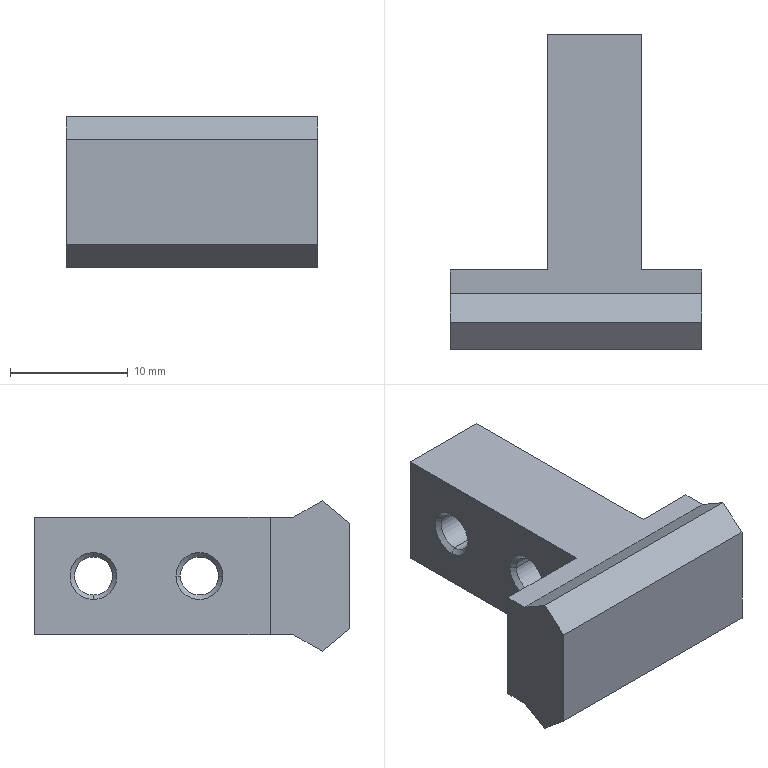Part | SolidWorks | features BaseBody 1 | 1 solid | 26 faces | box 21.4 x 26.74 x 12.8 mm | volume 3023 mm3 | plane 14 | cone 8 | cylinder 4 | commonest cylinder face diameters 3.242 x4
STEP:
#1=CARTESIAN_POINT('',(8.629,19.44,1.621));
#2=VERTEX_POINT('',#1);
#3=CARTESIAN_POINT('',(8.629,19.44,-1.621));
#4=VERTEX_POINT('',#3);
#5=CARTESIAN_POINT('',(8.629,19.44,0.));
#6=DIRECTION('',(1.,0.,0.));
#7=DIRECTION('',(0.,0.,-1.));
#8=AXIS2_PLACEMENT_3D('',#5,#6,#7);
#9=CIRCLE('',#8,1.621);
#10=EDGE_CURVE('',#2,#4,#9,.T.);
#11=ORIENTED_EDGE('',*,*,#10,.T.);
#12=CARTESIAN_POINT('',(8.25,19.44,-2.));
#13=VERTEX_POINT('',#12);
#14=CARTESIAN_POINT('',(8.25,19.44,-2.));
#15=DIRECTION('',(-0.7071,0.,-0.7071));
#16=VECTOR('',#15,1000.);
#17=LINE('',#14,#16);
#18=EDGE_CURVE('',#4,#13,#17,.T.);
#19=ORIENTED_EDGE('',*,*,#18,.T.);
#20=CARTESIAN_POINT('',(8.25,19.44,2.));
#21=VERTEX_POINT('',#20);
#22=CARTESIAN_POINT('',(8.25,19.44,0.));
#23=DIRECTION('',(1.,0.,0.));
#24=DIRECTION('',(0.,0.,-1.));
#25=AXIS2_PLACEMENT_3D('',#22,#23,#24);
#26=CIRCLE('',#25,2.);
#27=EDGE_CURVE('',#21,#13,#26,.T.);
#28=ORIENTED_EDGE('',*,*,#27,.F.);
#29=CARTESIAN_POINT('',(8.25,19.44,2.));
#30=DIRECTION('',(-0.7071,0.,0.7071));
#31=VECTOR('',#30,1000.);
#32=LINE('',#29,#31);
#33=EDGE_CURVE('',#2,#21,#32,.T.);
#34=ORIENTED_EDGE('',*,*,#33,.F.);
#35=EDGE_LOOP('',(#11,#19,#28,#34));
#36=FACE_OUTER_BOUND('',#35,.T.);
#37=CARTESIAN_POINT('',(8.25,19.44,0.));
#38=DIRECTION('',(-1.,0.,0.));
#39=DIRECTION('',(0.,0.,1.));
#40=AXIS2_PLACEMENT_3D('',#37,#38,#39);
#41=CONICAL_SURFACE('',#40,2.,0.7854);
#42=ADVANCED_FACE('',(#36),#41,.F.);
#43=ORIENTED_EDGE('',*,*,#10,.F.);
#44=CARTESIAN_POINT('',(15.871,19.44,1.621));
#45=VERTEX_POINT('',#44);
#46=CARTESIAN_POINT('',(16.25,19.44,1.621));
#47=DIRECTION('',(1.,0.,0.));
#48=VECTOR('',#47,1000.);
#49=LINE('',#46,#48);
#50=EDGE_CURVE('',#2,#45,#49,.T.);
#51=ORIENTED_EDGE('',*,*,#50,.T.);
#52=CARTESIAN_POINT('',(15.871,19.44,-1.621));
#53=VERTEX_POINT('',#52);
#54=CARTESIAN_POINT('',(15.871,19.44,0.));
#55=DIRECTION('',(1.,0.,0.));
#56=DIRECTION('',(0.,0.,-1.));
#57=AXIS2_PLACEMENT_3D('',#54,#55,#56);
#58=CIRCLE('',#57,1.621);
#59=EDGE_CURVE('',#45,#53,#58,.T.);
#60=ORIENTED_EDGE('',*,*,#59,.T.);
#61=CARTESIAN_POINT('',(16.25,19.44,-1.621));
#62=DIRECTION('',(1.,0.,0.));
#63=VECTOR('',#62,1000.);
#64=LINE('',#61,#63);
#65=EDGE_CURVE('',#4,#53,#64,.T.);
#66=ORIENTED_EDGE('',*,*,#65,.F.);
#67=EDGE_LOOP('',(#43,#51,#60,#66));
#68=FACE_OUTER_BOUND('',#67,.T.);
#69=CARTESIAN_POINT('',(16.25,19.44,0.));
#70=DIRECTION('',(1.,0.,0.));
#71=DIRECTION('',(0.,0.,-1.));
#72=AXIS2_PLACEMENT_3D('',#69,#70,#71);
#73=CYLINDRICAL_SURFACE('',#72,1.621);
#74=ADVANCED_FACE('',(#68),#73,.F.);
#75=ORIENTED_EDGE('',*,*,#59,.F.);
#76=CARTESIAN_POINT('',(16.25,19.44,2.));
#77=VERTEX_POINT('',#76);
#78=CARTESIAN_POINT('',(15.871,19.44,1.621));
#79=DIRECTION('',(0.7071,0.,0.7071));
#80=VECTOR('',#79,1000.);
#81=LINE('',#78,#80);
#82=EDGE_CURVE('',#45,#77,#81,.T.);
#83=ORIENTED_EDGE('',*,*,#82,.T.);
#84=CARTESIAN_POINT('',(16.25,19.44,-2.));
#85=VERTEX_POINT('',#84);
#86=CARTESIAN_POINT('',(16.25,19.44,0.));
#87=DIRECTION('',(1.,0.,0.));
#88=DIRECTION('',(0.,0.,-1.));
#89=AXIS2_PLACEMENT_3D('',#86,#87,#88);
#90=CIRCLE('',#89,2.);
#91=EDGE_CURVE('',#77,#85,#90,.T.);
#92=ORIENTED_EDGE('',*,*,#91,.T.);
#93=CARTESIAN_POINT('',(15.871,19.44,-1.621));
#94=DIRECTION('',(0.7071,0.,-0.7071));
#95=VECTOR('',#94,1000.);
#96=LINE('',#93,#95);
#97=EDGE_CURVE('',#53,#85,#96,.T.);
#98=ORIENTED_EDGE('',*,*,#97,.F.);
#99=EDGE_LOOP('',(#75,#83,#92,#98));
#100=FACE_OUTER_BOUND('',#99,.T.);
#101=CARTESIAN_POINT('',(15.871,19.44,0.));
#102=DIRECTION('',(1.,0.,0.));
#103=DIRECTION('',(0.,0.,-1.));
#104=AXIS2_PLACEMENT_3D('',#101,#102,#103);
#105=CONICAL_SURFACE('',#104,1.621,0.7854);
#106=ADVANCED_FACE('',(#100),#105,.F.);
#107=CARTESIAN_POINT('',(8.629,8.819,0.));
#108=VERTEX_POINT('',#107);
#109=CARTESIAN_POINT('',(8.629,12.061,0.));
#110=VERTEX_POINT('',#109);
#111=CARTESIAN_POINT('',(8.629,10.44,0.));
#112=DIRECTION('',(1.,0.,0.));
#113=DIRECTION('',(0.,1.,0.));
#114=AXIS2_PLACEMENT_3D('',#111,#112,#113);
#115=CIRCLE('',#114,1.621);
#116=EDGE_CURVE('',#108,#110,#115,.T.);
#117=ORIENTED_EDGE('',*,*,#116,.T.);
#118=CARTESIAN_POINT('',(8.25,12.44,0.));
#119=VERTEX_POINT('',#118);
#120=CARTESIAN_POINT('',(8.25,12.44,0.));
#121=DIRECTION('',(-0.7071,0.7071,0.));
#122=VECTOR('',#121,1000.);
#123=LINE('',#120,#122);
#124=EDGE_CURVE('',#110,#119,#123,.T.);
#125=ORIENTED_EDGE('',*,*,#124,.T.);
#126=CARTESIAN_POINT('',(8.25,8.44,0.));
#127=VERTEX_POINT('',#126);
#128=CARTESIAN_POINT('',(8.25,10.44,0.));
#129=DIRECTION('',(1.,0.,0.));
#130=DIRECTION('',(0.,1.,0.));
#131=AXIS2_PLACEMENT_3D('',#128,#129,#130);
#132=CIRCLE('',#131,2.);
#133=EDGE_CURVE('',#127,#119,#132,.T.);
#134=ORIENTED_EDGE('',*,*,#133,.F.);
#135=CARTESIAN_POINT('',(8.25,8.44,0.));
#136=DIRECTION('',(-0.7071,-0.7071,0.));
#137=VECTOR('',#136,1000.);
#138=LINE('',#135,#137);
#139=EDGE_CURVE('',#108,#127,#138,.T.);
#140=ORIENTED_EDGE('',*,*,#139,.F.);
#141=EDGE_LOOP('',(#117,#125,#134,#140));
#142=FACE_OUTER_BOUND('',#141,.T.);
#143=CARTESIAN_POINT('',(8.25,10.44,0.));
#144=DIRECTION('',(-1.,0.,0.));
#145=DIRECTION('',(0.,-1.,0.));
#146=AXIS2_PLACEMENT_3D('',#143,#144,#145);
#147=CONICAL_SURFACE('',#146,2.,0.7854);
#148=ADVANCED_FACE('',(#142),#147,.F.);
#149=ORIENTED_EDGE('',*,*,#116,.F.);
#150=CARTESIAN_POINT('',(15.871,8.819,0.));
#151=VERTEX_POINT('',#150);
#152=CARTESIAN_POINT('',(16.25,8.819,0.));
#153=DIRECTION('',(1.,0.,0.));
#154=VECTOR('',#153,1000.);
#155=LINE('',#152,#154);
#156=EDGE_CURVE('',#108,#151,#155,.T.);
#157=ORIENTED_EDGE('',*,*,#156,.T.);
#158=CARTESIAN_POINT('',(15.871,12.061,0.));
#159=VERTEX_POINT('',#158);
#160=CARTESIAN_POINT('',(15.871,10.44,0.));
#161=DIRECTION('',(1.,0.,0.));
#162=DIRECTION('',(0.,1.,0.));
#163=AXIS2_PLACEMENT_3D('',#160,#161,#162);
#164=CIRCLE('',#163,1.621);
#165=EDGE_CURVE('',#151,#159,#164,.T.);
#166=ORIENTED_EDGE('',*,*,#165,.T.);
#167=CARTESIAN_POINT('',(16.25,12.061,0.));
#168=DIRECTION('',(1.,0.,0.));
#169=VECTOR('',#168,1000.);
#170=LINE('',#167,#169);
#171=EDGE_CURVE('',#110,#159,#170,.T.);
#172=ORIENTED_EDGE('',*,*,#171,.F.);
#173=EDGE_LOOP('',(#149,#157,#166,#172));
#174=FACE_OUTER_BOUND('',#173,.T.);
#175=CARTESIAN_POINT('',(16.25,10.44,0.));
#176=DIRECTION('',(1.,0.,0.));
#177=DIRECTION('',(0.,1.,0.));
#178=AXIS2_PLACEMENT_3D('',#175,#176,#177);
#179=CYLINDRICAL_SURFACE('',#178,1.621);
#180=ADVANCED_FACE('',(#174),#179,.F.);
#181=ORIENTED_EDGE('',*,*,#165,.F.);
#182=CARTESIAN_POINT('',(16.25,8.44,0.));
#183=VERTEX_POINT('',#182);
#184=CARTESIAN_POINT('',(15.871,8.819,0.));
#185=DIRECTION('',(0.7071,-0.7071,0.));
#186=VECTOR('',#185,1000.);
#187=LINE('',#184,#186);
#188=EDGE_CURVE('',#151,#183,#187,.T.);
#189=ORIENTED_EDGE('',*,*,#188,.T.);
#190=CARTESIAN_POINT('',(16.25,12.44,0.));
#191=VERTEX_POINT('',#190);
#192=CARTESIAN_POINT('',(16.25,10.44,0.));
#193=DIRECTION('',(1.,0.,0.));
#194=DIRECTION('',(0.,1.,0.));
#195=AXIS2_PLACEMENT_3D('',#192,#193,#194);
#196=CIRCLE('',#195,2.);
#197=EDGE_CURVE('',#183,#191,#196,.T.);
#198=ORIENTED_EDGE('',*,*,#197,.T.);
#199=CARTESIAN_POINT('',(15.871,12.061,0.));
#200=DIRECTION('',(0.7071,0.7071,0.));
#201=VECTOR('',#200,1000.);
#202=LINE('',#199,#201);
#203=EDGE_CURVE('',#159,#191,#202,.T.);
#204=ORIENTED_EDGE('',*,*,#203,.F.);
#205=EDGE_LOOP('',(#181,#189,#198,#204));
#206=FACE_OUTER_BOUND('',#205,.T.);
#207=CARTESIAN_POINT('',(15.871,10.44,0.));
#208=DIRECTION('',(1.,0.,0.));
#209=DIRECTION('',(0.,1.,0.));
#210=AXIS2_PLACEMENT_3D('',#207,#208,#209);
#211=CONICAL_SURFACE('',#210,1.621,0.7854);
#212=ADVANCED_FACE('',(#206),#211,.F.);
#213=ORIENTED_EDGE('',*,*,#188,.F.);
#214=CARTESIAN_POINT('',(15.871,10.44,0.));
#215=DIRECTION('',(1.,0.,0.));
#216=DIRECTION('',(0.,1.,0.));
#217=AXIS2_PLACEMENT_3D('',#214,#215,#216);
#218=CIRCLE('',#217,1.621);
#219=EDGE_CURVE('',#159,#151,#218,.T.);
#220=ORIENTED_EDGE('',*,*,#219,.F.);
#221=ORIENTED_EDGE('',*,*,#203,.T.);
#222=CARTESIAN_POINT('',(16.25,10.44,0.));
#223=DIRECTION('',(1.,0.,0.));
#224=DIRECTION('',(0.,1.,0.));
#225=AXIS2_PLACEMENT_3D('',#222,#223,#224);
#226=CIRCLE('',#225,2.);
#227=EDGE_CURVE('',#191,#183,#226,.T.);
#228=ORIENTED_EDGE('',*,*,#227,.T.);
#229=EDGE_LOOP('',(#213,#220,#221,#228));
#230=FACE_OUTER_BOUND('',#229,.T.);
#231=CARTESIAN_POINT('',(15.871,10.44,0.));
#232=DIRECTION('',(1.,0.,0.));
#233=DIRECTION('',(0.,1.,0.));
#234=AXIS2_PLACEMENT_3D('',#231,#232,#233);
#235=CONICAL_SURFACE('',#234,1.621,0.7854);
#236=ADVANCED_FACE('',(#230),#235,.F.);
#237=ORIENTED_EDGE('',*,*,#156,.F.);
#238=CARTESIAN_POINT('',(8.629,10.44,0.));
#239=DIRECTION('',(1.,0.,0.));
#240=DIRECTION('',(0.,1.,0.));
#241=AXIS2_PLACEMENT_3D('',#238,#239,#240);
#242=CIRCLE('',#241,1.621);
#243=EDGE_CURVE('',#110,#108,#242,.T.);
#244=ORIENTED_EDGE('',*,*,#243,.F.);
#245=ORIENTED_EDGE('',*,*,#171,.T.);
#246=ORIENTED_EDGE('',*,*,#219,.T.);
#247=EDGE_LOOP('',(#237,#244,#245,#246));
#248=FACE_OUTER_BOUND('',#247,.T.);
#249=CARTESIAN_POINT('',(16.25,10.44,0.));
#250=DIRECTION('',(1.,0.,0.));
#251=DIRECTION('',(0.,1.,0.));
#252=AXIS2_PLACEMENT_3D('',#249,#250,#251);
#253=CYLINDRICAL_SURFACE('',#252,1.621);
#254=ADVANCED_FACE('',(#248),#253,.F.);
#255=ORIENTED_EDGE('',*,*,#124,.F.);
#256=ORIENTED_EDGE('',*,*,#243,.T.);
#257=ORIENTED_EDGE('',*,*,#139,.T.);
#258=CARTESIAN_POINT('',(8.25,10.44,0.));
#259=DIRECTION('',(1.,0.,0.));
#260=DIRECTION('',(0.,1.,0.));
#261=AXIS2_PLACEMENT_3D('',#258,#259,#260);
#262=CIRCLE('',#261,2.);
#263=EDGE_CURVE('',#119,#127,#262,.T.);
#264=ORIENTED_EDGE('',*,*,#263,.F.);
#265=EDGE_LOOP('',(#255,#256,#257,#264));
#266=FACE_OUTER_BOUND('',#265,.T.);
#267=CARTESIAN_POINT('',(8.25,10.44,0.));
#268=DIRECTION('',(-1.,0.,0.));
#269=DIRECTION('',(0.,-1.,0.));
#270=AXIS2_PLACEMENT_3D('',#267,#268,#269);
#271=CONICAL_SURFACE('',#270,2.,0.7854);
#272=ADVANCED_FACE('',(#266),#271,.F.);
#273=ORIENTED_EDGE('',*,*,#82,.F.);
#274=CARTESIAN_POINT('',(15.871,19.44,0.));
#275=DIRECTION('',(1.,0.,0.));
#276=DIRECTION('',(0.,0.,-1.));
#277=AXIS2_PLACEMENT_3D('',#274,#275,#276);
#278=CIRCLE('',#277,1.621);
#279=EDGE_CURVE('',#53,#45,#278,.T.);
#280=ORIENTED_EDGE('',*,*,#279,.F.);
#281=ORIENTED_EDGE('',*,*,#97,.T.);
#282=CARTESIAN_POINT('',(16.25,19.44,0.));
#283=DIRECTION('',(1.,0.,0.));
#284=DIRECTION('',(0.,0.,-1.));
#285=AXIS2_PLACEMENT_3D('',#282,#283,#284);
#286=CIRCLE('',#285,2.);
#287=EDGE_CURVE('',#85,#77,#286,.T.);
#288=ORIENTED_EDGE('',*,*,#287,.T.);
#289=EDGE_LOOP('',(#273,#280,#281,#288));
#290=FACE_OUTER_BOUND('',#289,.T.);
#291=CARTESIAN_POINT('',(15.871,19.44,0.));
#292=DIRECTION('',(1.,0.,0.));
#293=DIRECTION('',(0.,0.,-1.));
#294=AXIS2_PLACEMENT_3D('',#291,#292,#293);
#295=CONICAL_SURFACE('',#294,1.621,0.7854);
#296=ADVANCED_FACE('',(#290),#295,.F.);
#297=ORIENTED_EDGE('',*,*,#50,.F.);
#298=CARTESIAN_POINT('',(8.629,19.44,0.));
#299=DIRECTION('',(1.,0.,0.));
#300=DIRECTION('',(0.,0.,-1.));
#301=AXIS2_PLACEMENT_3D('',#298,#299,#300);
#302=CIRCLE('',#301,1.621);
#303=EDGE_CURVE('',#4,#2,#302,.T.);
#304=ORIENTED_EDGE('',*,*,#303,.F.);
#305=ORIENTED_EDGE('',*,*,#65,.T.);
#306=ORIENTED_EDGE('',*,*,#279,.T.);
#307=EDGE_LOOP('',(#297,#304,#305,#306));
#308=FACE_OUTER_BOUND('',#307,.T.);
#309=CARTESIAN_POINT('',(16.25,19.44,0.));
#310=DIRECTION('',(1.,0.,0.));
#311=DIRECTION('',(0.,0.,-1.));
#312=AXIS2_PLACEMENT_3D('',#309,#310,#311);
#313=CYLINDRICAL_SURFACE('',#312,1.621);
#314=ADVANCED_FACE('',(#308),#313,.F.);
#315=ORIENTED_EDGE('',*,*,#18,.F.);
#316=ORIENTED_EDGE('',*,*,#303,.T.);
#317=ORIENTED_EDGE('',*,*,#33,.T.);
#318=CARTESIAN_POINT('',(8.25,19.44,0.));
#319=DIRECTION('',(1.,0.,0.));
#320=DIRECTION('',(0.,0.,-1.));
#321=AXIS2_PLACEMENT_3D('',#318,#319,#320);
#322=CIRCLE('',#321,2.);
#323=EDGE_CURVE('',#13,#21,#322,.T.);
#324=ORIENTED_EDGE('',*,*,#323,.F.);
#325=EDGE_LOOP('',(#315,#316,#317,#324));
#326=FACE_OUTER_BOUND('',#325,.T.);
#327=CARTESIAN_POINT('',(8.25,19.44,0.));
#328=DIRECTION('',(-1.,0.,0.));
#329=DIRECTION('',(0.,0.,1.));
#330=AXIS2_PLACEMENT_3D('',#327,#328,#329);
#331=CONICAL_SURFACE('',#330,2.,0.7854);
#332=ADVANCED_FACE('',(#326),#331,.F.);
#333=CARTESIAN_POINT('',(8.25,24.44,-5.));
#334=VERTEX_POINT('',#333);
#335=CARTESIAN_POINT('',(8.25,24.44,5.));
#336=VERTEX_POINT('',#335);
#337=CARTESIAN_POINT('',(8.25,24.44,-5.));
#338=DIRECTION('',(0.,0.,1.));
#339=VECTOR('',#338,1000.);
#340=LINE('',#337,#339);
#341=EDGE_CURVE('',#334,#336,#340,.T.);
#342=ORIENTED_EDGE('',*,*,#341,.T.);
#343=CARTESIAN_POINT('',(16.25,24.44,5.));
#344=VERTEX_POINT('',#343);
#345=CARTESIAN_POINT('',(16.25,24.44,5.));
#346=DIRECTION('',(-1.,0.,0.));
#347=VECTOR('',#346,1000.);
#348=LINE('',#345,#347);
#349=EDGE_CURVE('',#344,#336,#348,.T.);
#350=ORIENTED_EDGE('',*,*,#349,.F.);
#351=CARTESIAN_POINT('',(16.25,24.44,-5.));
#352=VERTEX_POINT('',#351);
#353=CARTESIAN_POINT('',(16.25,24.44,-5.));
#354=DIRECTION('',(0.,0.,1.));
#355=VECTOR('',#354,1000.);
#356=LINE('',#353,#355);
#357=EDGE_CURVE('',#352,#344,#356,.T.);
#358=ORIENTED_EDGE('',*,*,#357,.F.);
#359=CARTESIAN_POINT('',(16.25,24.44,-5.));
#360=DIRECTION('',(-1.,0.,0.));
#361=VECTOR('',#360,1000.);
#362=LINE('',#359,#361);
#363=EDGE_CURVE('',#352,#334,#362,.T.);
#364=ORIENTED_EDGE('',*,*,#363,.T.);
#365=EDGE_LOOP('',(#342,#350,#358,#364));
#366=FACE_OUTER_BOUND('',#365,.T.);
#367=CARTESIAN_POINT('',(16.25,24.44,-5.));
#368=DIRECTION('',(0.,-1.,0.));
#369=DIRECTION('',(0.,0.,-1.));
#370=AXIS2_PLACEMENT_3D('',#367,#368,#369);
#371=PLANE('',#370);
#372=ADVANCED_FACE('',(#366),#371,.F.);
#373=CARTESIAN_POINT('',(8.25,4.44,-5.));
#374=VERTEX_POINT('',#373);
#375=CARTESIAN_POINT('',(8.25,0.,-5.));
#376=DIRECTION('',(0.,1.,0.));
#377=VECTOR('',#376,1000.);
#378=LINE('',#375,#377);
#379=EDGE_CURVE('',#374,#334,#378,.T.);
#380=ORIENTED_EDGE('',*,*,#379,.F.);
#381=CARTESIAN_POINT('',(8.25,4.44,5.));
#382=VERTEX_POINT('',#381);
#383=CARTESIAN_POINT('',(8.25,4.44,-5.));
#384=DIRECTION('',(0.,0.,1.));
#385=VECTOR('',#384,1000.);
#386=LINE('',#383,#385);
#387=EDGE_CURVE('',#374,#382,#386,.T.);
#388=ORIENTED_EDGE('',*,*,#387,.T.);
#389=CARTESIAN_POINT('',(8.25,24.44,5.));
#390=DIRECTION('',(0.,-1.,0.));
#391=VECTOR('',#390,1000.);
#392=LINE('',#389,#391);
#393=EDGE_CURVE('',#336,#382,#392,.T.);
#394=ORIENTED_EDGE('',*,*,#393,.F.);
#395=ORIENTED_EDGE('',*,*,#341,.F.);
#396=EDGE_LOOP('',(#380,#388,#394,#395));
#397=FACE_OUTER_BOUND('',#396,.T.);
#398=ORIENTED_EDGE('',*,*,#27,.T.);
#399=ORIENTED_EDGE('',*,*,#323,.T.);
#400=EDGE_LOOP('',(#398,#399));
#401=FACE_BOUND('',#400,.T.);
#402=ORIENTED_EDGE('',*,*,#133,.T.);
#403=ORIENTED_EDGE('',*,*,#263,.T.);
#404=EDGE_LOOP('',(#402,#403));
#405=FACE_BOUND('',#404,.T.);
#406=CARTESIAN_POINT('',(8.25,0.,0.));
#407=DIRECTION('',(1.,0.,0.));
#408=DIRECTION('',(0.,1.,0.));
#409=AXIS2_PLACEMENT_3D('',#406,#407,#408);
#410=PLANE('',#409);
#411=ADVANCED_FACE('',(#397,#401,#405),#410,.F.);
#412=CARTESIAN_POINT('',(16.25,4.44,-5.));
#413=VERTEX_POINT('',#412);
#414=CARTESIAN_POINT('',(16.25,4.44,5.));
#415=VERTEX_POINT('',#414);
#416=CARTESIAN_POINT('',(16.25,4.44,-5.));
#417=DIRECTION('',(0.,0.,1.));
#418=VECTOR('',#417,1000.);
#419=LINE('',#416,#418);
#420=EDGE_CURVE('',#413,#415,#419,.T.);
#421=ORIENTED_EDGE('',*,*,#420,.F.);
#422=CARTESIAN_POINT('',(16.25,0.,-5.));
#423=DIRECTION('',(0.,1.,0.));
#424=VECTOR('',#423,1000.);
#425=LINE('',#422,#424);
#426=EDGE_CURVE('',#413,#352,#425,.T.);
#427=ORIENTED_EDGE('',*,*,#426,.T.);
#428=ORIENTED_EDGE('',*,*,#357,.T.);
#429=CARTESIAN_POINT('',(16.25,24.44,5.));
#430=DIRECTION('',(0.,-1.,0.));
#431=VECTOR('',#430,1000.);
#432=LINE('',#429,#431);
#433=EDGE_CURVE('',#344,#415,#432,.T.);
#434=ORIENTED_EDGE('',*,*,#433,.T.);
#435=EDGE_LOOP('',(#421,#427,#428,#434));
#436=FACE_OUTER_BOUND('',#435,.T.);
#437=ORIENTED_EDGE('',*,*,#287,.F.);
#438=ORIENTED_EDGE('',*,*,#91,.F.);
#439=EDGE_LOOP('',(#437,#438));
#440=FACE_BOUND('',#439,.T.);
#441=ORIENTED_EDGE('',*,*,#227,.F.);
#442=ORIENTED_EDGE('',*,*,#197,.F.);
#443=EDGE_LOOP('',(#441,#442));
#444=FACE_BOUND('',#443,.T.);
#445=CARTESIAN_POINT('',(16.25,0.,0.));
#446=DIRECTION('',(1.,0.,0.));
#447=DIRECTION('',(0.,1.,0.));
#448=AXIS2_PLACEMENT_3D('',#445,#446,#447);
#449=PLANE('',#448);
#450=ADVANCED_FACE('',(#436,#440,#444),#449,.T.);
#451=CARTESIAN_POINT('',(0.,2.425,5.));
#452=VERTEX_POINT('',#451);
#453=CARTESIAN_POINT('',(0.,0.,6.4));
#454=VERTEX_POINT('',#453);
#455=CARTESIAN_POINT('',(0.,2.425,5.));
#456=DIRECTION('',(0.,-0.866,0.5));
#457=VECTOR('',#456,1000.);
#458=LINE('',#455,#457);
#459=EDGE_CURVE('',#452,#454,#458,.T.);
#460=ORIENTED_EDGE('',*,*,#459,.F.);
#461=CARTESIAN_POINT('',(0.,4.44,5.));
#462=VERTEX_POINT('',#461);
#463=CARTESIAN_POINT('',(0.,4.44,5.));
#464=DIRECTION('',(0.,-1.,0.));
#465=VECTOR('',#464,1000.);
#466=LINE('',#463,#465);
#467=EDGE_CURVE('',#462,#452,#466,.T.);
#468=ORIENTED_EDGE('',*,*,#467,.F.);
#469=CARTESIAN_POINT('',(0.,4.44,-5.));
#470=VERTEX_POINT('',#469);
#471=CARTESIAN_POINT('',(0.,4.44,-5.));
#472=DIRECTION('',(0.,0.,1.));
#473=VECTOR('',#472,1000.);
#474=LINE('',#471,#473);
#475=EDGE_CURVE('',#470,#462,#474,.T.);
#476=ORIENTED_EDGE('',*,*,#475,.F.);
#477=CARTESIAN_POINT('',(0.,2.425,-5.));
#478=VERTEX_POINT('',#477);
#479=CARTESIAN_POINT('',(0.,2.425,-5.));
#480=DIRECTION('',(0.,1.,0.));
#481=VECTOR('',#480,1000.);
#482=LINE('',#479,#481);
#483=EDGE_CURVE('',#478,#470,#482,.T.);
#484=ORIENTED_EDGE('',*,*,#483,.F.);
#485=CARTESIAN_POINT('',(0.,0.,-6.4));
#486=VERTEX_POINT('',#485);
#487=CARTESIAN_POINT('',(0.,0.,-6.4));
#488=DIRECTION('',(0.,0.866,0.5));
#489=VECTOR('',#488,1000.);
#490=LINE('',#487,#489);
#491=EDGE_CURVE('',#486,#478,#490,.T.);
#492=ORIENTED_EDGE('',*,*,#491,.F.);
#493=CARTESIAN_POINT('',(0.,-2.3,-4.47));
#494=VERTEX_POINT('',#493);
#495=CARTESIAN_POINT('',(0.,-2.3,-4.47));
#496=DIRECTION('',(0.,0.766,-0.6428));
#497=VECTOR('',#496,1000.);
#498=LINE('',#495,#497);
#499=EDGE_CURVE('',#494,#486,#498,.T.);
#500=ORIENTED_EDGE('',*,*,#499,.F.);
#501=CARTESIAN_POINT('',(0.,-2.3,4.47));
#502=VERTEX_POINT('',#501);
#503=CARTESIAN_POINT('',(0.,-2.3,4.47));
#504=DIRECTION('',(0.,0.,-1.));
#505=VECTOR('',#504,1000.);
#506=LINE('',#503,#505);
#507=EDGE_CURVE('',#502,#494,#506,.T.);
#508=ORIENTED_EDGE('',*,*,#507,.F.);
#509=CARTESIAN_POINT('',(0.,0.,6.4));
#510=DIRECTION('',(0.,-0.766,-0.6428));
#511=VECTOR('',#510,1000.);
#512=LINE('',#509,#511);
#513=EDGE_CURVE('',#454,#502,#512,.T.);
#514=ORIENTED_EDGE('',*,*,#513,.F.);
#515=EDGE_LOOP('',(#460,#468,#476,#484,#492,#500,#508,#514));
#516=FACE_OUTER_BOUND('',#515,.T.);
#517=CARTESIAN_POINT('',(0.,0.,0.));
#518=DIRECTION('',(1.,0.,0.));
#519=DIRECTION('',(0.,1.,0.));
#520=AXIS2_PLACEMENT_3D('',#517,#518,#519);
#521=PLANE('',#520);
#522=ADVANCED_FACE('',(#516),#521,.F.);
#523=CARTESIAN_POINT('',(21.4,2.425,5.));
#524=VERTEX_POINT('',#523);
#525=CARTESIAN_POINT('',(21.4,0.,6.4));
#526=VERTEX_POINT('',#525);
#527=CARTESIAN_POINT('',(21.4,2.425,5.));
#528=DIRECTION('',(0.,-0.866,0.5));
#529=VECTOR('',#528,1000.);
#530=LINE('',#527,#529);
#531=EDGE_CURVE('',#524,#526,#530,.T.);
#532=ORIENTED_EDGE('',*,*,#531,.T.);
#533=CARTESIAN_POINT('',(21.4,-2.3,4.47));
#534=VERTEX_POINT('',#533);
#535=CARTESIAN_POINT('',(21.4,0.,6.4));
#536=DIRECTION('',(0.,-0.766,-0.6428));
#537=VECTOR('',#536,1000.);
#538=LINE('',#535,#537);
#539=EDGE_CURVE('',#526,#534,#538,.T.);
#540=ORIENTED_EDGE('',*,*,#539,.T.);
#541=CARTESIAN_POINT('',(21.4,-2.3,-4.47));
#542=VERTEX_POINT('',#541);
#543=CARTESIAN_POINT('',(21.4,-2.3,4.47));
#544=DIRECTION('',(0.,0.,-1.));
#545=VECTOR('',#544,1000.);
#546=LINE('',#543,#545);
#547=EDGE_CURVE('',#534,#542,#546,.T.);
#548=ORIENTED_EDGE('',*,*,#547,.T.);
#549=CARTESIAN_POINT('',(21.4,0.,-6.4));
#550=VERTEX_POINT('',#549);
#551=CARTESIAN_POINT('',(21.4,-2.3,-4.47));
#552=DIRECTION('',(0.,0.766,-0.6428));
#553=VECTOR('',#552,1000.);
#554=LINE('',#551,#553);
#555=EDGE_CURVE('',#542,#550,#554,.T.);
#556=ORIENTED_EDGE('',*,*,#555,.T.);
#557=CARTESIAN_POINT('',(21.4,2.425,-5.));
#558=VERTEX_POINT('',#557);
#559=CARTESIAN_POINT('',(21.4,0.,-6.4));
#560=DIRECTION('',(0.,0.866,0.5));
#561=VECTOR('',#560,1000.);
#562=LINE('',#559,#561);
#563=EDGE_CURVE('',#550,#558,#562,.T.);
#564=ORIENTED_EDGE('',*,*,#563,.T.);
#565=CARTESIAN_POINT('',(21.4,4.44,-5.));
#566=VERTEX_POINT('',#565);
#567=CARTESIAN_POINT('',(21.4,2.425,-5.));
#568=DIRECTION('',(0.,1.,0.));
#569=VECTOR('',#568,1000.);
#570=LINE('',#567,#569);
#571=EDGE_CURVE('',#558,#566,#570,.T.);
#572=ORIENTED_EDGE('',*,*,#571,.T.);
#573=CARTESIAN_POINT('',(21.4,4.44,5.));
#574=VERTEX_POINT('',#573);
#575=CARTESIAN_POINT('',(21.4,4.44,-5.));
#576=DIRECTION('',(0.,0.,1.));
#577=VECTOR('',#576,1000.);
#578=LINE('',#575,#577);
#579=EDGE_CURVE('',#566,#574,#578,.T.);
#580=ORIENTED_EDGE('',*,*,#579,.T.);
#581=CARTESIAN_POINT('',(21.4,4.44,5.));
#582=DIRECTION('',(0.,-1.,0.));
#583=VECTOR('',#582,1000.);
#584=LINE('',#581,#583);
#585=EDGE_CURVE('',#574,#524,#584,.T.);
#586=ORIENTED_EDGE('',*,*,#585,.T.);
#587=EDGE_LOOP('',(#532,#540,#548,#556,#564,#572,#580,#586));
#588=FACE_OUTER_BOUND('',#587,.T.);
#589=CARTESIAN_POINT('',(21.4,0.,0.));
#590=DIRECTION('',(1.,0.,0.));
#591=DIRECTION('',(0.,1.,0.));
#592=AXIS2_PLACEMENT_3D('',#589,#590,#591);
#593=PLANE('',#592);
#594=ADVANCED_FACE('',(#588),#593,.T.);
#595=CARTESIAN_POINT('',(21.4,4.44,5.));
#596=DIRECTION('',(-1.,0.,0.));
#597=VECTOR('',#596,1000.);
#598=LINE('',#595,#597);
#599=EDGE_CURVE('',#574,#415,#598,.T.);
#600=ORIENTED_EDGE('',*,*,#599,.T.);
#601=ORIENTED_EDGE('',*,*,#433,.F.);
#602=ORIENTED_EDGE('',*,*,#349,.T.);
#603=ORIENTED_EDGE('',*,*,#393,.T.);
#604=CARTESIAN_POINT('',(21.4,4.44,5.));
#605=DIRECTION('',(-1.,0.,0.));
#606=VECTOR('',#605,1000.);
#607=LINE('',#604,#606);
#608=EDGE_CURVE('',#382,#462,#607,.T.);
#609=ORIENTED_EDGE('',*,*,#608,.T.);
#610=ORIENTED_EDGE('',*,*,#467,.T.);
#611=CARTESIAN_POINT('',(21.4,2.425,5.));
#612=DIRECTION('',(-1.,0.,0.));
#613=VECTOR('',#612,1000.);
#614=LINE('',#611,#613);
#615=EDGE_CURVE('',#524,#452,#614,.T.);
#616=ORIENTED_EDGE('',*,*,#615,.F.);
#617=ORIENTED_EDGE('',*,*,#585,.F.);
#618=EDGE_LOOP('',(#600,#601,#602,#603,#609,#610,#616,#617));
#619=FACE_OUTER_BOUND('',#618,.T.);
#620=CARTESIAN_POINT('',(21.4,4.44,5.));
#621=DIRECTION('',(0.,0.,-1.));
#622=DIRECTION('',(-1.,0.,0.));
#623=AXIS2_PLACEMENT_3D('',#620,#621,#622);
#624=PLANE('',#623);
#625=ADVANCED_FACE('',(#619),#624,.F.);
#626=CARTESIAN_POINT('',(21.4,4.44,-5.));
#627=DIRECTION('',(-1.,0.,0.));
#628=VECTOR('',#627,1000.);
#629=LINE('',#626,#628);
#630=EDGE_CURVE('',#566,#413,#629,.T.);
#631=ORIENTED_EDGE('',*,*,#630,.T.);
#632=ORIENTED_EDGE('',*,*,#420,.T.);
#633=ORIENTED_EDGE('',*,*,#599,.F.);
#634=ORIENTED_EDGE('',*,*,#579,.F.);
#635=EDGE_LOOP('',(#631,#632,#633,#634));
#636=FACE_OUTER_BOUND('',#635,.T.);
#637=CARTESIAN_POINT('',(21.4,4.44,-5.));
#638=DIRECTION('',(0.,-1.,0.));
#639=DIRECTION('',(0.,0.,-1.));
#640=AXIS2_PLACEMENT_3D('',#637,#638,#639);
#641=PLANE('',#640);
#642=ADVANCED_FACE('',(#636),#641,.F.);
#643=CARTESIAN_POINT('',(21.4,2.425,-5.));
#644=DIRECTION('',(-1.,0.,0.));
#645=VECTOR('',#644,1000.);
#646=LINE('',#643,#645);
#647=EDGE_CURVE('',#558,#478,#646,.T.);
#648=ORIENTED_EDGE('',*,*,#647,.T.);
#649=ORIENTED_EDGE('',*,*,#483,.T.);
#650=CARTESIAN_POINT('',(21.4,4.44,-5.));
#651=DIRECTION('',(-1.,0.,0.));
#652=VECTOR('',#651,1000.);
#653=LINE('',#650,#652);
#654=EDGE_CURVE('',#374,#470,#653,.T.);
#655=ORIENTED_EDGE('',*,*,#654,.F.);
#656=ORIENTED_EDGE('',*,*,#379,.T.);
#657=ORIENTED_EDGE('',*,*,#363,.F.);
#658=ORIENTED_EDGE('',*,*,#426,.F.);
#659=ORIENTED_EDGE('',*,*,#630,.F.);
#660=ORIENTED_EDGE('',*,*,#571,.F.);
#661=EDGE_LOOP('',(#648,#649,#655,#656,#657,#658,#659,#660));
#662=FACE_OUTER_BOUND('',#661,.T.);
#663=CARTESIAN_POINT('',(21.4,2.425,-5.));
#664=DIRECTION('',(0.,0.,1.));
#665=DIRECTION('',(0.,-1.,0.));
#666=AXIS2_PLACEMENT_3D('',#663,#664,#665);
#667=PLANE('',#666);
#668=ADVANCED_FACE('',(#662),#667,.F.);
#669=ORIENTED_EDGE('',*,*,#491,.T.);
#670=ORIENTED_EDGE('',*,*,#647,.F.);
#671=ORIENTED_EDGE('',*,*,#563,.F.);
#672=CARTESIAN_POINT('',(21.4,0.,-6.4));
#673=DIRECTION('',(-1.,0.,0.));
#674=VECTOR('',#673,1000.);
#675=LINE('',#672,#674);
#676=EDGE_CURVE('',#550,#486,#675,.T.);
#677=ORIENTED_EDGE('',*,*,#676,.T.);
#678=EDGE_LOOP('',(#669,#670,#671,#677));
#679=FACE_OUTER_BOUND('',#678,.T.);
#680=CARTESIAN_POINT('',(21.4,0.,-6.4));
#681=DIRECTION('',(0.,-0.5,0.866));
#682=DIRECTION('',(-1.,0.,0.));
#683=AXIS2_PLACEMENT_3D('',#680,#681,#682);
#684=PLANE('',#683);
#685=ADVANCED_FACE('',(#679),#684,.F.);
#686=ORIENTED_EDGE('',*,*,#499,.T.);
#687=ORIENTED_EDGE('',*,*,#676,.F.);
#688=ORIENTED_EDGE('',*,*,#555,.F.);
#689=CARTESIAN_POINT('',(21.4,-2.3,-4.47));
#690=DIRECTION('',(-1.,0.,0.));
#691=VECTOR('',#690,1000.);
#692=LINE('',#689,#691);
#693=EDGE_CURVE('',#542,#494,#692,.T.);
#694=ORIENTED_EDGE('',*,*,#693,.T.);
#695=EDGE_LOOP('',(#686,#687,#688,#694));
#696=FACE_OUTER_BOUND('',#695,.T.);
#697=CARTESIAN_POINT('',(21.4,-2.3,-4.47));
#698=DIRECTION('',(0.,0.6428,0.766));
#699=DIRECTION('',(1.,0.,0.));
#700=AXIS2_PLACEMENT_3D('',#697,#698,#699);
#701=PLANE('',#700);
#702=ADVANCED_FACE('',(#696),#701,.F.);
#703=ORIENTED_EDGE('',*,*,#507,.T.);
#704=ORIENTED_EDGE('',*,*,#693,.F.);
#705=ORIENTED_EDGE('',*,*,#547,.F.);
#706=CARTESIAN_POINT('',(21.4,-2.3,4.47));
#707=DIRECTION('',(-1.,0.,0.));
#708=VECTOR('',#707,1000.);
#709=LINE('',#706,#708);
#710=EDGE_CURVE('',#534,#502,#709,.T.);
#711=ORIENTED_EDGE('',*,*,#710,.T.);
#712=EDGE_LOOP('',(#703,#704,#705,#711));
#713=FACE_OUTER_BOUND('',#712,.T.);
#714=CARTESIAN_POINT('',(21.4,-2.3,4.47));
#715=DIRECTION('',(0.,1.,0.));
#716=DIRECTION('',(1.,0.,0.));
#717=AXIS2_PLACEMENT_3D('',#714,#715,#716);
#718=PLANE('',#717);
#719=ADVANCED_FACE('',(#713),#718,.F.);
#720=ORIENTED_EDGE('',*,*,#513,.T.);
#721=ORIENTED_EDGE('',*,*,#710,.F.);
#722=ORIENTED_EDGE('',*,*,#539,.F.);
#723=CARTESIAN_POINT('',(21.4,0.,6.4));
#724=DIRECTION('',(-1.,0.,0.));
#725=VECTOR('',#724,1000.);
#726=LINE('',#723,#725);
#727=EDGE_CURVE('',#526,#454,#726,.T.);
#728=ORIENTED_EDGE('',*,*,#727,.T.);
#729=EDGE_LOOP('',(#720,#721,#722,#728));
#730=FACE_OUTER_BOUND('',#729,.T.);
#731=CARTESIAN_POINT('',(21.4,0.,6.4));
#732=DIRECTION('',(0.,0.6428,-0.766));
#733=DIRECTION('',(-1.,0.,0.));
#734=AXIS2_PLACEMENT_3D('',#731,#732,#733);
#735=PLANE('',#734);
#736=ADVANCED_FACE('',(#730),#735,.F.);
#737=ORIENTED_EDGE('',*,*,#459,.T.);
#738=ORIENTED_EDGE('',*,*,#727,.F.);
#739=ORIENTED_EDGE('',*,*,#531,.F.);
#740=ORIENTED_EDGE('',*,*,#615,.T.);
#741=EDGE_LOOP('',(#737,#738,#739,#740));
#742=FACE_OUTER_BOUND('',#741,.T.);
#743=CARTESIAN_POINT('',(21.4,2.425,5.));
#744=DIRECTION('',(0.,-0.5,-0.866));
#745=DIRECTION('',(0.,-0.866,0.5));
#746=AXIS2_PLACEMENT_3D('',#743,#744,#745);
#747=PLANE('',#746);
#748=ADVANCED_FACE('',(#742),#747,.F.);
#749=ORIENTED_EDGE('',*,*,#387,.F.);
#750=ORIENTED_EDGE('',*,*,#654,.T.);
#751=ORIENTED_EDGE('',*,*,#475,.T.);
#752=ORIENTED_EDGE('',*,*,#608,.F.);
#753=EDGE_LOOP('',(#749,#750,#751,#752));
#754=FACE_OUTER_BOUND('',#753,.T.);
#755=CARTESIAN_POINT('',(21.4,4.44,-5.));
#756=DIRECTION('',(0.,-1.,0.));
#757=DIRECTION('',(0.,0.,-1.));
#758=AXIS2_PLACEMENT_3D('',#755,#756,#757);
#759=PLANE('',#758);
#760=ADVANCED_FACE('',(#754),#759,.F.);
#761=CLOSED_SHELL('',(#42,#74,#106,#148,#180,#212,#236,#254,#272,#296,#314,#332,#372,#411,#450,#522,#594,#625,#642,#668,#685,#702,#719,#736,#748,#760));
#762=MANIFOLD_SOLID_BREP('',#761);
#763=CARTESIAN_POINT('',(0.,0.,0.));
#764=DIRECTION('',(0.,0.,1.));
#765=DIRECTION('',(1.,0.,0.));
#766=AXIS2_PLACEMENT_3D('',#763,#764,#765);
#767=(LENGTH_UNIT()NAMED_UNIT(*)SI_UNIT(.MILLI.,.METRE.));
#768=UNCERTAINTY_MEASURE_WITH_UNIT(LENGTH_MEASURE(0.00001),#767,'','');
#769=(NAMED_UNIT(*)PLANE_ANGLE_UNIT()SI_UNIT($,.RADIAN.));
#770=(NAMED_UNIT(*)SI_UNIT($,.STERADIAN.)SOLID_ANGLE_UNIT());
#771=(GEOMETRIC_REPRESENTATION_CONTEXT(3)GLOBAL_UNCERTAINTY_ASSIGNED_CONTEXT((#768))GLOBAL_UNIT_ASSIGNED_CONTEXT((#767,#769,#770))REPRESENTATION_CONTEXT('',''));
#772=ADVANCED_BREP_SHAPE_REPRESENTATION('',(#762,#766),#771);